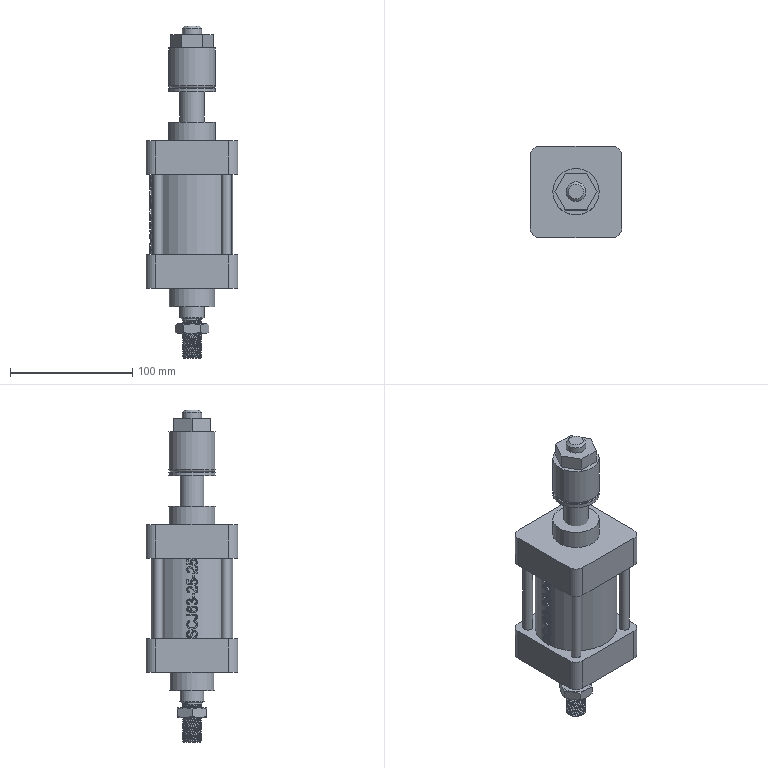Part | STEP file | YBQDJ-QD-11 | 2 solids | 169 faces | box 75 x 75 x 272 mm | volume 699847 mm3 | plane 57 | spline 45 | cylinder 41 | cone 25 | torus 1 | commonest cylinder face diameters 16 x11 69 x11 6.8 x4 8 x4 67 x4 38 x3